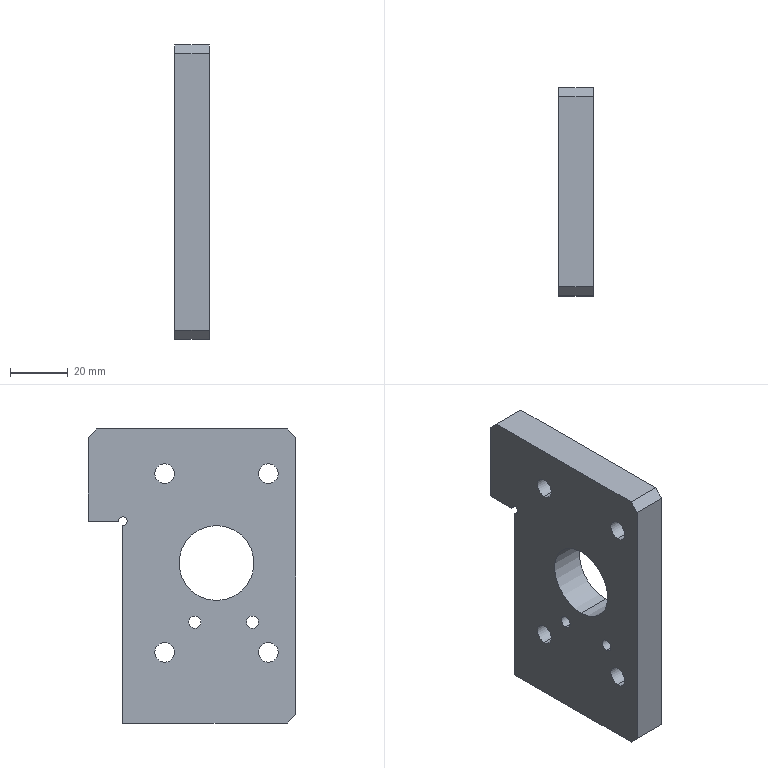Part | SolidWorks | features HoleWzd 3, Cut 2, Chamfer 1, Extrusion 1 | 1 solid | 34 faces | box 12 x 72 x 102 mm | volume 69020 mm3 | cylinder 19 | plane 11 | cone 4 | commonest cylinder face diameters 4.2 x8 6.8 x8 26 x2 3 x1
STEP:
#1=CARTESIAN_POINT('',(6.,47.6,-94.1));
#2=VERTEX_POINT('',#1);
#3=CARTESIAN_POINT('',(6.,47.6,-89.9));
#4=VERTEX_POINT('',#3);
#5=CARTESIAN_POINT('',(6.,47.6,-92.));
#6=DIRECTION('',(0.,1.,0.));
#7=DIRECTION('',(0.,0.,1.));
#8=AXIS2_PLACEMENT_3D('',#5,#6,#7);
#9=CIRCLE('',#8,2.1);
#10=EDGE_CURVE('',#2,#4,#9,.T.);
#11=ORIENTED_EDGE('',*,*,#10,.F.);
#12=CARTESIAN_POINT('',(6.,60.,-94.1));
#13=VERTEX_POINT('',#12);
#14=CARTESIAN_POINT('',(6.,60.,-94.1));
#15=DIRECTION('',(0.,1.,0.));
#16=VECTOR('',#15,1000.);
#17=LINE('',#14,#16);
#18=EDGE_CURVE('',#2,#13,#17,.T.);
#19=ORIENTED_EDGE('',*,*,#18,.T.);
#20=CARTESIAN_POINT('',(6.,60.,-89.9));
#21=VERTEX_POINT('',#20);
#22=CARTESIAN_POINT('',(6.,60.,-92.));
#23=DIRECTION('',(0.,1.,0.));
#24=DIRECTION('',(0.,0.,1.));
#25=AXIS2_PLACEMENT_3D('',#22,#23,#24);
#26=CIRCLE('',#25,2.1);
#27=EDGE_CURVE('',#13,#21,#26,.T.);
#28=ORIENTED_EDGE('',*,*,#27,.T.);
#29=CARTESIAN_POINT('',(6.,60.,-89.9));
#30=DIRECTION('',(0.,1.,0.));
#31=VECTOR('',#30,1000.);
#32=LINE('',#29,#31);
#33=EDGE_CURVE('',#4,#21,#32,.T.);
#34=ORIENTED_EDGE('',*,*,#33,.F.);
#35=EDGE_LOOP('',(#11,#19,#28,#34));
#36=FACE_OUTER_BOUND('',#35,.T.);
#37=CARTESIAN_POINT('',(6.,60.,-92.));
#38=DIRECTION('',(0.,1.,0.));
#39=DIRECTION('',(0.,0.,1.));
#40=AXIS2_PLACEMENT_3D('',#37,#38,#39);
#41=CYLINDRICAL_SURFACE('',#40,2.1);
#42=ADVANCED_FACE('',(#36),#41,.F.);
#43=CARTESIAN_POINT('',(6.,46.338,-92.));
#44=VERTEX_POINT('',#43);
#45=CARTESIAN_POINT('',(6.,47.6,-89.9));
#46=DIRECTION('',(0.,0.515,0.8572));
#47=VECTOR('',#46,1000.);
#48=LINE('',#45,#47);
#49=EDGE_CURVE('',#44,#4,#48,.T.);
#50=ORIENTED_EDGE('',*,*,#49,.F.);
#51=CARTESIAN_POINT('',(6.,47.6,-94.1));
#52=DIRECTION('',(0.,0.515,-0.8572));
#53=VECTOR('',#52,1000.);
#54=LINE('',#51,#53);
#55=EDGE_CURVE('',#44,#2,#54,.T.);
#56=ORIENTED_EDGE('',*,*,#55,.T.);
#57=ORIENTED_EDGE('',*,*,#10,.T.);
#58=EDGE_LOOP('',(#50,#56,#57));
#59=FACE_OUTER_BOUND('',#58,.T.);
#60=CARTESIAN_POINT('',(6.,47.6,-92.));
#61=DIRECTION('',(0.,1.,0.));
#62=DIRECTION('',(0.,0.,1.));
#63=AXIS2_PLACEMENT_3D('',#60,#61,#62);
#64=CONICAL_SURFACE('',#63,2.1,1.03);
#65=ADVANCED_FACE('',(#59),#64,.F.);
#66=CARTESIAN_POINT('',(6.,47.6,-44.1));
#67=VERTEX_POINT('',#66);
#68=CARTESIAN_POINT('',(6.,47.6,-39.9));
#69=VERTEX_POINT('',#68);
#70=CARTESIAN_POINT('',(6.,47.6,-42.));
#71=DIRECTION('',(0.,1.,0.));
#72=DIRECTION('',(0.,0.,1.));
#73=AXIS2_PLACEMENT_3D('',#70,#71,#72);
#74=CIRCLE('',#73,2.1);
#75=EDGE_CURVE('',#67,#69,#74,.T.);
#76=ORIENTED_EDGE('',*,*,#75,.F.);
#77=CARTESIAN_POINT('',(6.,60.,-44.1));
#78=VERTEX_POINT('',#77);
#79=CARTESIAN_POINT('',(6.,60.,-44.1));
#80=DIRECTION('',(0.,1.,0.));
#81=VECTOR('',#80,1000.);
#82=LINE('',#79,#81);
#83=EDGE_CURVE('',#67,#78,#82,.T.);
#84=ORIENTED_EDGE('',*,*,#83,.T.);
#85=CARTESIAN_POINT('',(6.,60.,-39.9));
#86=VERTEX_POINT('',#85);
#87=CARTESIAN_POINT('',(6.,60.,-42.));
#88=DIRECTION('',(0.,1.,0.));
#89=DIRECTION('',(0.,0.,1.));
#90=AXIS2_PLACEMENT_3D('',#87,#88,#89);
#91=CIRCLE('',#90,2.1);
#92=EDGE_CURVE('',#78,#86,#91,.T.);
#93=ORIENTED_EDGE('',*,*,#92,.T.);
#94=CARTESIAN_POINT('',(6.,60.,-39.9));
#95=DIRECTION('',(0.,1.,0.));
#96=VECTOR('',#95,1000.);
#97=LINE('',#94,#96);
#98=EDGE_CURVE('',#69,#86,#97,.T.);
#99=ORIENTED_EDGE('',*,*,#98,.F.);
#100=EDGE_LOOP('',(#76,#84,#93,#99));
#101=FACE_OUTER_BOUND('',#100,.T.);
#102=CARTESIAN_POINT('',(6.,60.,-42.));
#103=DIRECTION('',(0.,1.,0.));
#104=DIRECTION('',(0.,0.,1.));
#105=AXIS2_PLACEMENT_3D('',#102,#103,#104);
#106=CYLINDRICAL_SURFACE('',#105,2.1);
#107=ADVANCED_FACE('',(#101),#106,.F.);
#108=CARTESIAN_POINT('',(6.,46.338,-42.));
#109=VERTEX_POINT('',#108);
#110=CARTESIAN_POINT('',(6.,47.6,-39.9));
#111=DIRECTION('',(0.,0.515,0.8572));
#112=VECTOR('',#111,1000.);
#113=LINE('',#110,#112);
#114=EDGE_CURVE('',#109,#69,#113,.T.);
#115=ORIENTED_EDGE('',*,*,#114,.F.);
#116=CARTESIAN_POINT('',(6.,47.6,-44.1));
#117=DIRECTION('',(0.,0.515,-0.8572));
#118=VECTOR('',#117,1000.);
#119=LINE('',#116,#118);
#120=EDGE_CURVE('',#109,#67,#119,.T.);
#121=ORIENTED_EDGE('',*,*,#120,.T.);
#122=ORIENTED_EDGE('',*,*,#75,.T.);
#123=EDGE_LOOP('',(#115,#121,#122));
#124=FACE_OUTER_BOUND('',#123,.T.);
#125=CARTESIAN_POINT('',(6.,47.6,-42.));
#126=DIRECTION('',(0.,1.,0.));
#127=DIRECTION('',(0.,0.,1.));
#128=AXIS2_PLACEMENT_3D('',#125,#126,#127);
#129=CONICAL_SURFACE('',#128,2.1,1.03);
#130=ADVANCED_FACE('',(#124),#129,.F.);
#131=CARTESIAN_POINT('',(0.,35.,-64.9));
#132=VERTEX_POINT('',#131);
#133=CARTESIAN_POINT('',(0.,35.,-69.1));
#134=VERTEX_POINT('',#133);
#135=CARTESIAN_POINT('',(0.,35.,-67.));
#136=DIRECTION('',(1.,0.,0.));
#137=DIRECTION('',(0.,0.,-1.));
#138=AXIS2_PLACEMENT_3D('',#135,#136,#137);
#139=CIRCLE('',#138,2.1);
#140=EDGE_CURVE('',#132,#134,#139,.T.);
#141=ORIENTED_EDGE('',*,*,#140,.F.);
#142=CARTESIAN_POINT('',(12.,35.,-64.9));
#143=VERTEX_POINT('',#142);
#144=CARTESIAN_POINT('',(12.,35.,-64.9));
#145=DIRECTION('',(1.,0.,0.));
#146=VECTOR('',#145,1000.);
#147=LINE('',#144,#146);
#148=EDGE_CURVE('',#132,#143,#147,.T.);
#149=ORIENTED_EDGE('',*,*,#148,.T.);
#150=CARTESIAN_POINT('',(12.,35.,-69.1));
#151=VERTEX_POINT('',#150);
#152=CARTESIAN_POINT('',(12.,35.,-67.));
#153=DIRECTION('',(1.,0.,0.));
#154=DIRECTION('',(0.,0.,-1.));
#155=AXIS2_PLACEMENT_3D('',#152,#153,#154);
#156=CIRCLE('',#155,2.1);
#157=EDGE_CURVE('',#143,#151,#156,.T.);
#158=ORIENTED_EDGE('',*,*,#157,.T.);
#159=CARTESIAN_POINT('',(12.,35.,-69.1));
#160=DIRECTION('',(1.,0.,0.));
#161=VECTOR('',#160,1000.);
#162=LINE('',#159,#161);
#163=EDGE_CURVE('',#134,#151,#162,.T.);
#164=ORIENTED_EDGE('',*,*,#163,.F.);
#165=EDGE_LOOP('',(#141,#149,#158,#164));
#166=FACE_OUTER_BOUND('',#165,.T.);
#167=CARTESIAN_POINT('',(12.,35.,-67.));
#168=DIRECTION('',(1.,0.,0.));
#169=DIRECTION('',(0.,0.,-1.));
#170=AXIS2_PLACEMENT_3D('',#167,#168,#169);
#171=CYLINDRICAL_SURFACE('',#170,2.1);
#172=ADVANCED_FACE('',(#166),#171,.F.);
#173=CARTESIAN_POINT('',(0.,15.,-64.9));
#174=VERTEX_POINT('',#173);
#175=CARTESIAN_POINT('',(0.,15.,-69.1));
#176=VERTEX_POINT('',#175);
#177=CARTESIAN_POINT('',(0.,15.,-67.));
#178=DIRECTION('',(1.,0.,0.));
#179=DIRECTION('',(0.,0.,-1.));
#180=AXIS2_PLACEMENT_3D('',#177,#178,#179);
#181=CIRCLE('',#180,2.1);
#182=EDGE_CURVE('',#174,#176,#181,.T.);
#183=ORIENTED_EDGE('',*,*,#182,.F.);
#184=CARTESIAN_POINT('',(12.,15.,-64.9));
#185=VERTEX_POINT('',#184);
#186=CARTESIAN_POINT('',(12.,15.,-64.9));
#187=DIRECTION('',(1.,0.,0.));
#188=VECTOR('',#187,1000.);
#189=LINE('',#186,#188);
#190=EDGE_CURVE('',#174,#185,#189,.T.);
#191=ORIENTED_EDGE('',*,*,#190,.T.);
#192=CARTESIAN_POINT('',(12.,15.,-69.1));
#193=VERTEX_POINT('',#192);
#194=CARTESIAN_POINT('',(12.,15.,-67.));
#195=DIRECTION('',(1.,0.,0.));
#196=DIRECTION('',(0.,0.,-1.));
#197=AXIS2_PLACEMENT_3D('',#194,#195,#196);
#198=CIRCLE('',#197,2.1);
#199=EDGE_CURVE('',#185,#193,#198,.T.);
#200=ORIENTED_EDGE('',*,*,#199,.T.);
#201=CARTESIAN_POINT('',(12.,15.,-69.1));
#202=DIRECTION('',(1.,0.,0.));
#203=VECTOR('',#202,1000.);
#204=LINE('',#201,#203);
#205=EDGE_CURVE('',#176,#193,#204,.T.);
#206=ORIENTED_EDGE('',*,*,#205,.F.);
#207=EDGE_LOOP('',(#183,#191,#200,#206));
#208=FACE_OUTER_BOUND('',#207,.T.);
#209=CARTESIAN_POINT('',(12.,15.,-67.));
#210=DIRECTION('',(1.,0.,0.));
#211=DIRECTION('',(0.,0.,-1.));
#212=AXIS2_PLACEMENT_3D('',#209,#210,#211);
#213=CYLINDRICAL_SURFACE('',#212,2.1);
#214=ADVANCED_FACE('',(#208),#213,.F.);
#215=CARTESIAN_POINT('',(12.,45.5,-74.1));
#216=VERTEX_POINT('',#215);
#217=CARTESIAN_POINT('',(12.,45.5,-80.9));
#218=VERTEX_POINT('',#217);
#219=CARTESIAN_POINT('',(12.,45.5,-77.5));
#220=DIRECTION('',(1.,0.,0.));
#221=DIRECTION('',(0.,0.,-1.));
#222=AXIS2_PLACEMENT_3D('',#219,#220,#221);
#223=CIRCLE('',#222,3.4);
#224=EDGE_CURVE('',#216,#218,#223,.T.);
#225=ORIENTED_EDGE('',*,*,#224,.T.);
#226=CARTESIAN_POINT('',(0.,45.5,-80.9));
#227=VERTEX_POINT('',#226);
#228=CARTESIAN_POINT('',(0.,45.5,-80.9));
#229=DIRECTION('',(-1.,0.,0.));
#230=VECTOR('',#229,1000.);
#231=LINE('',#228,#230);
#232=EDGE_CURVE('',#218,#227,#231,.T.);
#233=ORIENTED_EDGE('',*,*,#232,.T.);
#234=CARTESIAN_POINT('',(0.,45.5,-74.1));
#235=VERTEX_POINT('',#234);
#236=CARTESIAN_POINT('',(0.,45.5,-77.5));
#237=DIRECTION('',(-1.,0.,0.));
#238=DIRECTION('',(0.,0.,1.));
#239=AXIS2_PLACEMENT_3D('',#236,#237,#238);
#240=CIRCLE('',#239,3.4);
#241=EDGE_CURVE('',#227,#235,#240,.T.);
#242=ORIENTED_EDGE('',*,*,#241,.T.);
#243=CARTESIAN_POINT('',(0.,45.5,-74.1));
#244=DIRECTION('',(-1.,0.,0.));
#245=VECTOR('',#244,1000.);
#246=LINE('',#243,#245);
#247=EDGE_CURVE('',#216,#235,#246,.T.);
#248=ORIENTED_EDGE('',*,*,#247,.F.);
#249=EDGE_LOOP('',(#225,#233,#242,#248));
#250=FACE_OUTER_BOUND('',#249,.T.);
#251=CARTESIAN_POINT('',(0.,45.5,-77.5));
#252=DIRECTION('',(-1.,0.,0.));
#253=DIRECTION('',(0.,0.,1.));
#254=AXIS2_PLACEMENT_3D('',#251,#252,#253);
#255=CYLINDRICAL_SURFACE('',#254,3.4);
#256=ADVANCED_FACE('',(#250),#255,.F.);
#257=CARTESIAN_POINT('',(12.,9.5,-74.1));
#258=VERTEX_POINT('',#257);
#259=CARTESIAN_POINT('',(12.,9.5,-80.9));
#260=VERTEX_POINT('',#259);
#261=CARTESIAN_POINT('',(12.,9.5,-77.5));
#262=DIRECTION('',(1.,0.,0.));
#263=DIRECTION('',(0.,0.,-1.));
#264=AXIS2_PLACEMENT_3D('',#261,#262,#263);
#265=CIRCLE('',#264,3.4);
#266=EDGE_CURVE('',#258,#260,#265,.T.);
#267=ORIENTED_EDGE('',*,*,#266,.T.);
#268=CARTESIAN_POINT('',(0.,9.5,-80.9));
#269=VERTEX_POINT('',#268);
#270=CARTESIAN_POINT('',(0.,9.5,-80.9));
#271=DIRECTION('',(-1.,0.,0.));
#272=VECTOR('',#271,1000.);
#273=LINE('',#270,#272);
#274=EDGE_CURVE('',#260,#269,#273,.T.);
#275=ORIENTED_EDGE('',*,*,#274,.T.);
#276=CARTESIAN_POINT('',(0.,9.5,-74.1));
#277=VERTEX_POINT('',#276);
#278=CARTESIAN_POINT('',(0.,9.5,-77.5));
#279=DIRECTION('',(-1.,0.,0.));
#280=DIRECTION('',(0.,0.,1.));
#281=AXIS2_PLACEMENT_3D('',#278,#279,#280);
#282=CIRCLE('',#281,3.4);
#283=EDGE_CURVE('',#269,#277,#282,.T.);
#284=ORIENTED_EDGE('',*,*,#283,.T.);
#285=CARTESIAN_POINT('',(0.,9.5,-74.1));
#286=DIRECTION('',(-1.,0.,0.));
#287=VECTOR('',#286,1000.);
#288=LINE('',#285,#287);
#289=EDGE_CURVE('',#258,#277,#288,.T.);
#290=ORIENTED_EDGE('',*,*,#289,.F.);
#291=EDGE_LOOP('',(#267,#275,#284,#290));
#292=FACE_OUTER_BOUND('',#291,.T.);
#293=CARTESIAN_POINT('',(0.,9.5,-77.5));
#294=DIRECTION('',(-1.,0.,0.));
#295=DIRECTION('',(0.,0.,1.));
#296=AXIS2_PLACEMENT_3D('',#293,#294,#295);
#297=CYLINDRICAL_SURFACE('',#296,3.4);
#298=ADVANCED_FACE('',(#292),#297,.F.);
#299=CARTESIAN_POINT('',(12.,9.5,-12.1));
#300=VERTEX_POINT('',#299);
#301=CARTESIAN_POINT('',(12.,9.5,-18.9));
#302=VERTEX_POINT('',#301);
#303=CARTESIAN_POINT('',(12.,9.5,-15.5));
#304=DIRECTION('',(1.,0.,0.));
#305=DIRECTION('',(0.,0.,-1.));
#306=AXIS2_PLACEMENT_3D('',#303,#304,#305);
#307=CIRCLE('',#306,3.4);
#308=EDGE_CURVE('',#300,#302,#307,.T.);
#309=ORIENTED_EDGE('',*,*,#308,.T.);
#310=CARTESIAN_POINT('',(0.,9.5,-18.9));
#311=VERTEX_POINT('',#310);
#312=CARTESIAN_POINT('',(0.,9.5,-18.9));
#313=DIRECTION('',(-1.,0.,0.));
#314=VECTOR('',#313,1000.);
#315=LINE('',#312,#314);
#316=EDGE_CURVE('',#302,#311,#315,.T.);
#317=ORIENTED_EDGE('',*,*,#316,.T.);
#318=CARTESIAN_POINT('',(0.,9.5,-12.1));
#319=VERTEX_POINT('',#318);
#320=CARTESIAN_POINT('',(0.,9.5,-15.5));
#321=DIRECTION('',(-1.,0.,0.));
#322=DIRECTION('',(0.,0.,1.));
#323=AXIS2_PLACEMENT_3D('',#320,#321,#322);
#324=CIRCLE('',#323,3.4);
#325=EDGE_CURVE('',#311,#319,#324,.T.);
#326=ORIENTED_EDGE('',*,*,#325,.T.);
#327=CARTESIAN_POINT('',(0.,9.5,-12.1));
#328=DIRECTION('',(-1.,0.,0.));
#329=VECTOR('',#328,1000.);
#330=LINE('',#327,#329);
#331=EDGE_CURVE('',#300,#319,#330,.T.);
#332=ORIENTED_EDGE('',*,*,#331,.F.);
#333=EDGE_LOOP('',(#309,#317,#326,#332));
#334=FACE_OUTER_BOUND('',#333,.T.);
#335=CARTESIAN_POINT('',(0.,9.5,-15.5));
#336=DIRECTION('',(-1.,0.,0.));
#337=DIRECTION('',(0.,0.,1.));
#338=AXIS2_PLACEMENT_3D('',#335,#336,#337);
#339=CYLINDRICAL_SURFACE('',#338,3.4);
#340=ADVANCED_FACE('',(#334),#339,.F.);
#341=CARTESIAN_POINT('',(12.,45.5,-12.1));
#342=VERTEX_POINT('',#341);
#343=CARTESIAN_POINT('',(12.,45.5,-18.9));
#344=VERTEX_POINT('',#343);
#345=CARTESIAN_POINT('',(12.,45.5,-15.5));
#346=DIRECTION('',(1.,0.,0.));
#347=DIRECTION('',(0.,0.,-1.));
#348=AXIS2_PLACEMENT_3D('',#345,#346,#347);
#349=CIRCLE('',#348,3.4);
#350=EDGE_CURVE('',#342,#344,#349,.T.);
#351=ORIENTED_EDGE('',*,*,#350,.T.);
#352=CARTESIAN_POINT('',(0.,45.5,-18.9));
#353=VERTEX_POINT('',#352);
#354=CARTESIAN_POINT('',(0.,45.5,-18.9));
#355=DIRECTION('',(-1.,0.,0.));
#356=VECTOR('',#355,1000.);
#357=LINE('',#354,#356);
#358=EDGE_CURVE('',#344,#353,#357,.T.);
#359=ORIENTED_EDGE('',*,*,#358,.T.);
#360=CARTESIAN_POINT('',(0.,45.5,-12.1));
#361=VERTEX_POINT('',#360);
#362=CARTESIAN_POINT('',(0.,45.5,-15.5));
#363=DIRECTION('',(-1.,0.,0.));
#364=DIRECTION('',(0.,0.,1.));
#365=AXIS2_PLACEMENT_3D('',#362,#363,#364);
#366=CIRCLE('',#365,3.4);
#367=EDGE_CURVE('',#353,#361,#366,.T.);
#368=ORIENTED_EDGE('',*,*,#367,.T.);
#369=CARTESIAN_POINT('',(0.,45.5,-12.1));
#370=DIRECTION('',(-1.,0.,0.));
#371=VECTOR('',#370,1000.);
#372=LINE('',#369,#371);
#373=EDGE_CURVE('',#342,#361,#372,.T.);
#374=ORIENTED_EDGE('',*,*,#373,.F.);
#375=EDGE_LOOP('',(#351,#359,#368,#374));
#376=FACE_OUTER_BOUND('',#375,.T.);
#377=CARTESIAN_POINT('',(0.,45.5,-15.5));
#378=DIRECTION('',(-1.,0.,0.));
#379=DIRECTION('',(0.,0.,1.));
#380=AXIS2_PLACEMENT_3D('',#377,#378,#379);
#381=CYLINDRICAL_SURFACE('',#380,3.4);
#382=ADVANCED_FACE('',(#376),#381,.F.);
#383=CARTESIAN_POINT('',(0.,27.5,-33.5));
#384=VERTEX_POINT('',#383);
#385=CARTESIAN_POINT('',(0.,27.5,-59.5));
#386=VERTEX_POINT('',#385);
#387=CARTESIAN_POINT('',(0.,27.5,-46.5));
#388=DIRECTION('',(1.,0.,0.));
#389=DIRECTION('',(0.,0.,-1.));
#390=AXIS2_PLACEMENT_3D('',#387,#388,#389);
#391=CIRCLE('',#390,13.);
#392=EDGE_CURVE('',#384,#386,#391,.T.);
#393=ORIENTED_EDGE('',*,*,#392,.F.);
#394=CARTESIAN_POINT('',(12.,27.5,-33.5));
#395=VERTEX_POINT('',#394);
#396=CARTESIAN_POINT('',(0.,27.5,-33.5));
#397=DIRECTION('',(1.,0.,0.));
#398=VECTOR('',#397,1000.);
#399=LINE('',#396,#398);
#400=EDGE_CURVE('',#384,#395,#399,.T.);
#401=ORIENTED_EDGE('',*,*,#400,.T.);
#402=CARTESIAN_POINT('',(12.,27.5,-59.5));
#403=VERTEX_POINT('',#402);
#404=CARTESIAN_POINT('',(12.,27.5,-46.5));
#405=DIRECTION('',(1.,0.,0.));
#406=DIRECTION('',(0.,0.,-1.));
#407=AXIS2_PLACEMENT_3D('',#404,#405,#406);
#408=CIRCLE('',#407,13.);
#409=EDGE_CURVE('',#395,#403,#408,.T.);
#410=ORIENTED_EDGE('',*,*,#409,.T.);
#411=CARTESIAN_POINT('',(0.,27.5,-59.5));
#412=DIRECTION('',(1.,0.,0.));
#413=VECTOR('',#412,1000.);
#414=LINE('',#411,#413);
#415=EDGE_CURVE('',#386,#403,#414,.T.);
#416=ORIENTED_EDGE('',*,*,#415,.F.);
#417=EDGE_LOOP('',(#393,#401,#410,#416));
#418=FACE_OUTER_BOUND('',#417,.T.);
#419=CARTESIAN_POINT('',(0.,27.5,-46.5));
#420=DIRECTION('',(1.,0.,0.));
#421=DIRECTION('',(0.,0.,-1.));
#422=AXIS2_PLACEMENT_3D('',#419,#420,#421);
#423=CYLINDRICAL_SURFACE('',#422,13.);
#424=ADVANCED_FACE('',(#418),#423,.F.);
#425=CARTESIAN_POINT('',(12.,69.,0.));
#426=VERTEX_POINT('',#425);
#427=CARTESIAN_POINT('',(12.,3.,0.));
#428=VERTEX_POINT('',#427);
#429=CARTESIAN_POINT('',(12.,72.,0.));
#430=DIRECTION('',(0.,-1.,0.));
#431=VECTOR('',#430,1000.);
#432=LINE('',#429,#431);
#433=EDGE_CURVE('',#426,#428,#432,.T.);
#434=ORIENTED_EDGE('',*,*,#433,.F.);
#435=CARTESIAN_POINT('',(0.,69.,0.));
#436=VERTEX_POINT('',#435);
#437=CARTESIAN_POINT('',(12.,69.,0.));
#438=DIRECTION('',(-1.,0.,0.));
#439=VECTOR('',#438,1000.);
#440=LINE('',#437,#439);
#441=EDGE_CURVE('',#426,#436,#440,.T.);
#442=ORIENTED_EDGE('',*,*,#441,.T.);
#443=CARTESIAN_POINT('',(0.,3.,0.));
#444=VERTEX_POINT('',#443);
#445=CARTESIAN_POINT('',(0.,72.,0.));
#446=DIRECTION('',(0.,-1.,0.));
#447=VECTOR('',#446,1000.);
#448=LINE('',#445,#447);
#449=EDGE_CURVE('',#436,#444,#448,.T.);
#450=ORIENTED_EDGE('',*,*,#449,.T.);
#451=CARTESIAN_POINT('',(12.,3.,0.));
#452=DIRECTION('',(1.,0.,0.));
#453=VECTOR('',#452,1000.);
#454=LINE('',#451,#453);
#455=EDGE_CURVE('',#444,#428,#454,.T.);
#456=ORIENTED_EDGE('',*,*,#455,.T.);
#457=EDGE_LOOP('',(#434,#442,#450,#456));
#458=FACE_OUTER_BOUND('',#457,.T.);
#459=CARTESIAN_POINT('',(12.,72.,0.));
#460=DIRECTION('',(0.,0.,-1.));
#461=DIRECTION('',(0.,1.,0.));
#462=AXIS2_PLACEMENT_3D('',#459,#460,#461);
#463=PLANE('',#462);
#464=ADVANCED_FACE('',(#458),#463,.F.);
#465=CARTESIAN_POINT('',(0.,0.,-3.));
#466=VERTEX_POINT('',#465);
#467=CARTESIAN_POINT('',(0.,0.,-99.));
#468=VERTEX_POINT('',#467);
#469=CARTESIAN_POINT('',(0.,0.,0.));
#470=DIRECTION('',(0.,0.,-1.));
#471=VECTOR('',#470,1000.);
#472=LINE('',#469,#471);
#473=EDGE_CURVE('',#466,#468,#472,.T.);
#474=ORIENTED_EDGE('',*,*,#473,.T.);
#475=CARTESIAN_POINT('',(12.,0.,-99.));
#476=VERTEX_POINT('',#475);
#477=CARTESIAN_POINT('',(12.,0.,-99.));
#478=DIRECTION('',(1.,0.,0.));
#479=VECTOR('',#478,1000.);
#480=LINE('',#477,#479);
#481=EDGE_CURVE('',#468,#476,#480,.T.);
#482=ORIENTED_EDGE('',*,*,#481,.T.);
#483=CARTESIAN_POINT('',(12.,0.,-3.));
#484=VERTEX_POINT('',#483);
#485=CARTESIAN_POINT('',(12.,0.,0.));
#486=DIRECTION('',(0.,0.,-1.));
#487=VECTOR('',#486,1000.);
#488=LINE('',#485,#487);
#489=EDGE_CURVE('',#484,#476,#488,.T.);
#490=ORIENTED_EDGE('',*,*,#489,.F.);
#491=CARTESIAN_POINT('',(12.,0.,-3.));
#492=DIRECTION('',(-1.,0.,0.));
#493=VECTOR('',#492,1000.);
#494=LINE('',#491,#493);
#495=EDGE_CURVE('',#484,#466,#494,.T.);
#496=ORIENTED_EDGE('',*,*,#495,.T.);
#497=EDGE_LOOP('',(#474,#482,#490,#496));
#498=FACE_OUTER_BOUND('',#497,.T.);
#499=CARTESIAN_POINT('',(12.,0.,0.));
#500=DIRECTION('',(0.,1.,0.));
#501=DIRECTION('',(0.,0.,1.));
#502=AXIS2_PLACEMENT_3D('',#499,#500,#501);
#503=PLANE('',#502);
#504=ADVANCED_FACE('',(#498),#503,.F.);
#505=CARTESIAN_POINT('',(12.,3.,-102.));
#506=VERTEX_POINT('',#505);
#507=CARTESIAN_POINT('',(12.,60.,-102.));
#508=VERTEX_POINT('',#507);
#509=CARTESIAN_POINT('',(12.,0.,-102.));
#510=DIRECTION('',(0.,1.,0.));
#511=VECTOR('',#510,1000.);
#512=LINE('',#509,#511);
#513=EDGE_CURVE('',#506,#508,#512,.T.);
#514=ORIENTED_EDGE('',*,*,#513,.F.);
#515=CARTESIAN_POINT('',(0.,3.,-102.));
#516=VERTEX_POINT('',#515);
#517=CARTESIAN_POINT('',(12.,3.,-102.));
#518=DIRECTION('',(-1.,0.,0.));
#519=VECTOR('',#518,1000.);
#520=LINE('',#517,#519);
#521=EDGE_CURVE('',#506,#516,#520,.T.);
#522=ORIENTED_EDGE('',*,*,#521,.T.);
#523=CARTESIAN_POINT('',(0.,60.,-102.));
#524=VERTEX_POINT('',#523);
#525=CARTESIAN_POINT('',(0.,0.,-102.));
#526=DIRECTION('',(0.,1.,0.));
#527=VECTOR('',#526,1000.);
#528=LINE('',#525,#527);
#529=EDGE_CURVE('',#516,#524,#528,.T.);
#530=ORIENTED_EDGE('',*,*,#529,.T.);
#531=CARTESIAN_POINT('',(12.,60.,-102.));
#532=DIRECTION('',(-1.,0.,0.));
#533=VECTOR('',#532,1000.);
#534=LINE('',#531,#533);
#535=EDGE_CURVE('',#508,#524,#534,.T.);
#536=ORIENTED_EDGE('',*,*,#535,.F.);
#537=EDGE_LOOP('',(#514,#522,#530,#536));
#538=FACE_OUTER_BOUND('',#537,.T.);
#539=CARTESIAN_POINT('',(12.,0.,-102.));
#540=DIRECTION('',(0.,0.,1.));
#541=DIRECTION('',(1.,0.,0.));
#542=AXIS2_PLACEMENT_3D('',#539,#540,#541);
#543=PLANE('',#542);
#544=ADVANCED_FACE('',(#538),#543,.F.);
#545=CARTESIAN_POINT('',(6.,60.,-92.));
#546=DIRECTION('',(0.,1.,0.));
#547=DIRECTION('',(0.,0.,1.));
#548=AXIS2_PLACEMENT_3D('',#545,#546,#547);
#549=CIRCLE('',#548,2.1);
#550=EDGE_CURVE('',#21,#13,#549,.T.);
#551=ORIENTED_EDGE('',*,*,#550,.F.);
#552=ORIENTED_EDGE('',*,*,#27,.F.);
#553=EDGE_LOOP('',(#551,#552));
#554=FACE_BOUND('',#553,.T.);
#555=CARTESIAN_POINT('',(6.,60.,-42.));
#556=DIRECTION('',(0.,1.,0.));
#557=DIRECTION('',(0.,0.,1.));
#558=AXIS2_PLACEMENT_3D('',#555,#556,#557);
#559=CIRCLE('',#558,2.1);
#560=EDGE_CURVE('',#86,#78,#559,.T.);
#561=ORIENTED_EDGE('',*,*,#560,.F.);
#562=ORIENTED_EDGE('',*,*,#92,.F.);
#563=EDGE_LOOP('',(#561,#562));
#564=FACE_BOUND('',#563,.T.);
#565=CARTESIAN_POINT('',(0.,60.,-33.5));
#566=VERTEX_POINT('',#565);
#567=CARTESIAN_POINT('',(0.,60.,-102.));
#568=DIRECTION('',(0.,0.,1.));
#569=VECTOR('',#568,1000.);
#570=LINE('',#567,#569);
#571=EDGE_CURVE('',#524,#566,#570,.T.);
#572=ORIENTED_EDGE('',*,*,#571,.T.);
#573=CARTESIAN_POINT('',(12.,60.,-33.5));
#574=VERTEX_POINT('',#573);
#575=CARTESIAN_POINT('',(0.,60.,-33.5));
#576=DIRECTION('',(1.,0.,0.));
#577=VECTOR('',#576,1000.);
#578=LINE('',#575,#577);
#579=EDGE_CURVE('',#566,#574,#578,.T.);
#580=ORIENTED_EDGE('',*,*,#579,.T.);
#581=CARTESIAN_POINT('',(12.,60.,-102.));
#582=DIRECTION('',(0.,0.,1.));
#583=VECTOR('',#582,1000.);
#584=LINE('',#581,#583);
#585=EDGE_CURVE('',#508,#574,#584,.T.);
#586=ORIENTED_EDGE('',*,*,#585,.F.);
#587=ORIENTED_EDGE('',*,*,#535,.T.);
#588=EDGE_LOOP('',(#572,#580,#586,#587));
#589=FACE_OUTER_BOUND('',#588,.T.);
#590=CARTESIAN_POINT('',(12.,60.,-102.));
#591=DIRECTION('',(0.,-1.,0.));
#592=DIRECTION('',(0.,0.,-1.));
#593=AXIS2_PLACEMENT_3D('',#590,#591,#592);
#594=PLANE('',#593);
#595=ADVANCED_FACE('',(#554,#564,#589),#594,.F.);
#596=CARTESIAN_POINT('',(12.,61.5,-32.));
#597=VERTEX_POINT('',#596);
#598=CARTESIAN_POINT('',(12.,72.,-32.));
#599=VERTEX_POINT('',#598);
#600=CARTESIAN_POINT('',(12.,60.,-32.));
#601=DIRECTION('',(0.,1.,0.));
#602=VECTOR('',#601,1000.);
#603=LINE('',#600,#602);
#604=EDGE_CURVE('',#597,#599,#603,.T.);
#605=ORIENTED_EDGE('',*,*,#604,.F.);
#606=CARTESIAN_POINT('',(0.,61.5,-32.));
#607=VERTEX_POINT('',#606);
#608=CARTESIAN_POINT('',(0.,61.5,-32.));
#609=DIRECTION('',(-1.,0.,0.));
#610=VECTOR('',#609,1000.);
#611=LINE('',#608,#610);
#612=EDGE_CURVE('',#597,#607,#611,.T.);
#613=ORIENTED_EDGE('',*,*,#612,.T.);
#614=CARTESIAN_POINT('',(0.,72.,-32.));
#615=VERTEX_POINT('',#614);
#616=CARTESIAN_POINT('',(0.,60.,-32.));
#617=DIRECTION('',(0.,1.,0.));
#618=VECTOR('',#617,1000.);
#619=LINE('',#616,#618);
#620=EDGE_CURVE('',#607,#615,#619,.T.);
#621=ORIENTED_EDGE('',*,*,#620,.T.);
#622=CARTESIAN_POINT('',(12.,72.,-32.));
#623=DIRECTION('',(-1.,0.,0.));
#624=VECTOR('',#623,1000.);
#625=LINE('',#622,#624);
#626=EDGE_CURVE('',#599,#615,#625,.T.);
#627=ORIENTED_EDGE('',*,*,#626,.F.);
#628=EDGE_LOOP('',(#605,#613,#621,#627));
#629=FACE_OUTER_BOUND('',#628,.T.);
#630=CARTESIAN_POINT('',(12.,60.,-32.));
#631=DIRECTION('',(0.,0.,1.));
#632=DIRECTION('',(1.,0.,0.));
#633=AXIS2_PLACEMENT_3D('',#630,#631,#632);
#634=PLANE('',#633);
#635=ADVANCED_FACE('',(#629),#634,.F.);
#636=CARTESIAN_POINT('',(0.,72.,-3.));
#637=VERTEX_POINT('',#636);
#638=CARTESIAN_POINT('',(0.,72.,-32.));
#639=DIRECTION('',(0.,0.,1.));
#640=VECTOR('',#639,1000.);
#641=LINE('',#638,#640);
#642=EDGE_CURVE('',#615,#637,#641,.T.);
#643=ORIENTED_EDGE('',*,*,#642,.T.);
#644=CARTESIAN_POINT('',(12.,72.,-3.));
#645=VERTEX_POINT('',#644);
#646=CARTESIAN_POINT('',(12.,72.,-3.));
#647=DIRECTION('',(1.,0.,0.));
#648=VECTOR('',#647,1000.);
#649=LINE('',#646,#648);
#650=EDGE_CURVE('',#637,#645,#649,.T.);
#651=ORIENTED_EDGE('',*,*,#650,.T.);
#652=CARTESIAN_POINT('',(12.,72.,-32.));
#653=DIRECTION('',(0.,0.,1.));
#654=VECTOR('',#653,1000.);
#655=LINE('',#652,#654);
#656=EDGE_CURVE('',#599,#645,#655,.T.);
#657=ORIENTED_EDGE('',*,*,#656,.F.);
#658=ORIENTED_EDGE('',*,*,#626,.T.);
#659=EDGE_LOOP('',(#643,#651,#657,#658));
#660=FACE_OUTER_BOUND('',#659,.T.);
#661=CARTESIAN_POINT('',(12.,72.,-32.));
#662=DIRECTION('',(0.,-1.,0.));
#663=DIRECTION('',(0.,0.,-1.));
#664=AXIS2_PLACEMENT_3D('',#661,#662,#663);
#665=PLANE('',#664);
#666=ADVANCED_FACE('',(#660),#665,.F.);
#667=CARTESIAN_POINT('',(12.,60.,-32.));
#668=DIRECTION('',(1.,0.,0.));
#669=DIRECTION('',(0.,0.,-1.));
#670=AXIS2_PLACEMENT_3D('',#667,#668,#669);
#671=CIRCLE('',#670,1.5);
#672=EDGE_CURVE('',#597,#574,#671,.T.);
#673=ORIENTED_EDGE('',*,*,#672,.F.);
#674=ORIENTED_EDGE('',*,*,#604,.T.);
#675=ORIENTED_EDGE('',*,*,#656,.T.);
#676=CARTESIAN_POINT('',(12.,34.5,34.5));
#677=DIRECTION('',(0.,-0.7071,0.7071));
#678=VECTOR('',#677,1000.);
#679=LINE('',#676,#678);
#680=EDGE_CURVE('',#645,#426,#679,.T.);
#681=ORIENTED_EDGE('',*,*,#680,.T.);
#682=ORIENTED_EDGE('',*,*,#433,.T.);
#683=CARTESIAN_POINT('',(12.,1.5,-1.5));
#684=DIRECTION('',(0.,-0.7071,-0.7071));
#685=VECTOR('',#684,1000.);
#686=LINE('',#683,#685);
#687=EDGE_CURVE('',#428,#484,#686,.T.);
#688=ORIENTED_EDGE('',*,*,#687,.T.);
#689=ORIENTED_EDGE('',*,*,#489,.T.);
#690=CARTESIAN_POINT('',(12.,-49.5,-49.5));
#691=DIRECTION('',(0.,0.7071,-0.7071));
#692=VECTOR('',#691,1000.);
#693=LINE('',#690,#692);
#694=EDGE_CURVE('',#476,#506,#693,.T.);
#695=ORIENTED_EDGE('',*,*,#694,.T.);
#696=ORIENTED_EDGE('',*,*,#513,.T.);
#697=ORIENTED_EDGE('',*,*,#585,.T.);
#698=EDGE_LOOP('',(#673,#674,#675,#681,#682,#688,#689,#695,#696,#697));
#699=FACE_OUTER_BOUND('',#698,.T.);
#700=CARTESIAN_POINT('',(12.,35.,-67.));
#701=DIRECTION('',(1.,0.,0.));
#702=DIRECTION('',(0.,0.,-1.));
#703=AXIS2_PLACEMENT_3D('',#700,#701,#702);
#704=CIRCLE('',#703,2.1);
#705=EDGE_CURVE('',#151,#143,#704,.T.);
#706=ORIENTED_EDGE('',*,*,#705,.F.);
#707=ORIENTED_EDGE('',*,*,#157,.F.);
#708=EDGE_LOOP('',(#706,#707));
#709=FACE_BOUND('',#708,.T.);
#710=CARTESIAN_POINT('',(12.,15.,-67.));
#711=DIRECTION('',(1.,0.,0.));
#712=DIRECTION('',(0.,0.,-1.));
#713=AXIS2_PLACEMENT_3D('',#710,#711,#712);
#714=CIRCLE('',#713,2.1);
#715=EDGE_CURVE('',#193,#185,#714,.T.);
#716=ORIENTED_EDGE('',*,*,#715,.F.);
#717=ORIENTED_EDGE('',*,*,#199,.F.);
#718=EDGE_LOOP('',(#716,#717));
#719=FACE_BOUND('',#718,.T.);
#720=ORIENTED_EDGE('',*,*,#224,.F.);
#721=CARTESIAN_POINT('',(12.,45.5,-77.5));
#722=DIRECTION('',(1.,0.,0.));
#723=DIRECTION('',(0.,0.,-1.));
#724=AXIS2_PLACEMENT_3D('',#721,#722,#723);
#725=CIRCLE('',#724,3.4);
#726=EDGE_CURVE('',#218,#216,#725,.T.);
#727=ORIENTED_EDGE('',*,*,#726,.F.);
#728=EDGE_LOOP('',(#720,#727));
#729=FACE_BOUND('',#728,.T.);
#730=ORIENTED_EDGE('',*,*,#266,.F.);
#731=CARTESIAN_POINT('',(12.,9.5,-77.5));
#732=DIRECTION('',(1.,0.,0.));
#733=DIRECTION('',(0.,0.,-1.));
#734=AXIS2_PLACEMENT_3D('',#731,#732,#733);
#735=CIRCLE('',#734,3.4);
#736=EDGE_CURVE('',#260,#258,#735,.T.);
#737=ORIENTED_EDGE('',*,*,#736,.F.);
#738=EDGE_LOOP('',(#730,#737));
#739=FACE_BOUND('',#738,.T.);
#740=ORIENTED_EDGE('',*,*,#308,.F.);
#741=CARTESIAN_POINT('',(12.,9.5,-15.5));
#742=DIRECTION('',(1.,0.,0.));
#743=DIRECTION('',(0.,0.,-1.));
#744=AXIS2_PLACEMENT_3D('',#741,#742,#743);
#745=CIRCLE('',#744,3.4);
#746=EDGE_CURVE('',#302,#300,#745,.T.);
#747=ORIENTED_EDGE('',*,*,#746,.F.);
#748=EDGE_LOOP('',(#740,#747));
#749=FACE_BOUND('',#748,.T.);
#750=ORIENTED_EDGE('',*,*,#350,.F.);
#751=CARTESIAN_POINT('',(12.,45.5,-15.5));
#752=DIRECTION('',(1.,0.,0.));
#753=DIRECTION('',(0.,0.,-1.));
#754=AXIS2_PLACEMENT_3D('',#751,#752,#753);
#755=CIRCLE('',#754,3.4);
#756=EDGE_CURVE('',#344,#342,#755,.T.);
#757=ORIENTED_EDGE('',*,*,#756,.F.);
#758=EDGE_LOOP('',(#750,#757));
#759=FACE_BOUND('',#758,.T.);
#760=CARTESIAN_POINT('',(12.,27.5,-46.5));
#761=DIRECTION('',(1.,0.,0.));
#762=DIRECTION('',(0.,0.,-1.));
#763=AXIS2_PLACEMENT_3D('',#760,#761,#762);
#764=CIRCLE('',#763,13.);
#765=EDGE_CURVE('',#403,#395,#764,.T.);
#766=ORIENTED_EDGE('',*,*,#765,.F.);
#767=ORIENTED_EDGE('',*,*,#409,.F.);
#768=EDGE_LOOP('',(#766,#767));
#769=FACE_BOUND('',#768,.T.);
#770=CARTESIAN_POINT('',(12.,0.,0.));
#771=DIRECTION('',(1.,0.,0.));
#772=DIRECTION('',(0.,0.,-1.));
#773=AXIS2_PLACEMENT_3D('',#770,#771,#772);
#774=PLANE('',#773);
#775=ADVANCED_FACE('',(#699,#709,#719,#729,#739,#749,#759,#769),#774,.T.);
#776=CARTESIAN_POINT('',(0.,35.,-67.));
#777=DIRECTION('',(1.,0.,0.));
#778=DIRECTION('',(0.,0.,-1.));
#779=AXIS2_PLACEMENT_3D('',#776,#777,#778);
#780=CIRCLE('',#779,2.1);
#781=EDGE_CURVE('',#134,#132,#780,.T.);
#782=ORIENTED_EDGE('',*,*,#781,.T.);
#783=ORIENTED_EDGE('',*,*,#140,.T.);
#784=EDGE_LOOP('',(#782,#783));
#785=FACE_BOUND('',#784,.T.);
#786=CARTESIAN_POINT('',(0.,15.,-67.));
#787=DIRECTION('',(1.,0.,0.));
#788=DIRECTION('',(0.,0.,-1.));
#789=AXIS2_PLACEMENT_3D('',#786,#787,#788);
#790=CIRCLE('',#789,2.1);
#791=EDGE_CURVE('',#176,#174,#790,.T.);
#792=ORIENTED_EDGE('',*,*,#791,.T.);
#793=ORIENTED_EDGE('',*,*,#182,.T.);
#794=EDGE_LOOP('',(#792,#793));
#795=FACE_BOUND('',#794,.T.);
#796=CARTESIAN_POINT('',(0.,45.5,-77.5));
#797=DIRECTION('',(-1.,0.,0.));
#798=DIRECTION('',(0.,0.,1.));
#799=AXIS2_PLACEMENT_3D('',#796,#797,#798);
#800=CIRCLE('',#799,3.4);
#801=EDGE_CURVE('',#235,#227,#800,.T.);
#802=ORIENTED_EDGE('',*,*,#801,.F.);
#803=ORIENTED_EDGE('',*,*,#241,.F.);
#804=EDGE_LOOP('',(#802,#803));
#805=FACE_BOUND('',#804,.T.);
#806=CARTESIAN_POINT('',(0.,9.5,-77.5));
#807=DIRECTION('',(-1.,0.,0.));
#808=DIRECTION('',(0.,0.,1.));
#809=AXIS2_PLACEMENT_3D('',#806,#807,#808);
#810=CIRCLE('',#809,3.4);
#811=EDGE_CURVE('',#277,#269,#810,.T.);
#812=ORIENTED_EDGE('',*,*,#811,.F.);
#813=ORIENTED_EDGE('',*,*,#283,.F.);
#814=EDGE_LOOP('',(#812,#813));
#815=FACE_BOUND('',#814,.T.);
#816=CARTESIAN_POINT('',(0.,9.5,-15.5));
#817=DIRECTION('',(-1.,0.,0.));
#818=DIRECTION('',(0.,0.,1.));
#819=AXIS2_PLACEMENT_3D('',#816,#817,#818);
#820=CIRCLE('',#819,3.4);
#821=EDGE_CURVE('',#319,#311,#820,.T.);
#822=ORIENTED_EDGE('',*,*,#821,.F.);
#823=ORIENTED_EDGE('',*,*,#325,.F.);
#824=EDGE_LOOP('',(#822,#823));
#825=FACE_BOUND('',#824,.T.);
#826=CARTESIAN_POINT('',(0.,45.5,-15.5));
#827=DIRECTION('',(-1.,0.,0.));
#828=DIRECTION('',(0.,0.,1.));
#829=AXIS2_PLACEMENT_3D('',#826,#827,#828);
#830=CIRCLE('',#829,3.4);
#831=EDGE_CURVE('',#361,#353,#830,.T.);
#832=ORIENTED_EDGE('',*,*,#831,.F.);
#833=ORIENTED_EDGE('',*,*,#367,.F.);
#834=EDGE_LOOP('',(#832,#833));
#835=FACE_BOUND('',#834,.T.);
#836=CARTESIAN_POINT('',(0.,27.5,-46.5));
#837=DIRECTION('',(1.,0.,0.));
#838=DIRECTION('',(0.,0.,-1.));
#839=AXIS2_PLACEMENT_3D('',#836,#837,#838);
#840=CIRCLE('',#839,13.);
#841=EDGE_CURVE('',#386,#384,#840,.T.);
#842=ORIENTED_EDGE('',*,*,#841,.T.);
#843=ORIENTED_EDGE('',*,*,#392,.T.);
#844=EDGE_LOOP('',(#842,#843));
#845=FACE_BOUND('',#844,.T.);
#846=ORIENTED_EDGE('',*,*,#620,.F.);
#847=CARTESIAN_POINT('',(0.,60.,-32.));
#848=DIRECTION('',(1.,0.,0.));
#849=DIRECTION('',(0.,0.,-1.));
#850=AXIS2_PLACEMENT_3D('',#847,#848,#849);
#851=CIRCLE('',#850,1.5);
#852=EDGE_CURVE('',#607,#566,#851,.T.);
#853=ORIENTED_EDGE('',*,*,#852,.T.);
#854=ORIENTED_EDGE('',*,*,#571,.F.);
#855=ORIENTED_EDGE('',*,*,#529,.F.);
#856=CARTESIAN_POINT('',(0.,3.,-102.));
#857=DIRECTION('',(0.,-0.7071,0.7071));
#858=VECTOR('',#857,1000.);
#859=LINE('',#856,#858);
#860=EDGE_CURVE('',#516,#468,#859,.T.);
#861=ORIENTED_EDGE('',*,*,#860,.T.);
#862=ORIENTED_EDGE('',*,*,#473,.F.);
#863=CARTESIAN_POINT('',(0.,0.,-3.));
#864=DIRECTION('',(0.,0.7071,0.7071));
#865=VECTOR('',#864,1000.);
#866=LINE('',#863,#865);
#867=EDGE_CURVE('',#466,#444,#866,.T.);
#868=ORIENTED_EDGE('',*,*,#867,.T.);
#869=ORIENTED_EDGE('',*,*,#449,.F.);
#870=CARTESIAN_POINT('',(0.,69.,0.));
#871=DIRECTION('',(0.,0.7071,-0.7071));
#872=VECTOR('',#871,1000.);
#873=LINE('',#870,#872);
#874=EDGE_CURVE('',#436,#637,#873,.T.);
#875=ORIENTED_EDGE('',*,*,#874,.T.);
#876=ORIENTED_EDGE('',*,*,#642,.F.);
#877=EDGE_LOOP('',(#846,#853,#854,#855,#861,#862,#868,#869,#875,#876));
#878=FACE_OUTER_BOUND('',#877,.T.);
#879=CARTESIAN_POINT('',(0.,0.,0.));
#880=DIRECTION('',(1.,0.,0.));
#881=DIRECTION('',(0.,0.,-1.));
#882=AXIS2_PLACEMENT_3D('',#879,#880,#881);
#883=PLANE('',#882);
#884=ADVANCED_FACE('',(#785,#795,#805,#815,#825,#835,#845,#878),#883,.F.);
#885=ORIENTED_EDGE('',*,*,#400,.F.);
#886=ORIENTED_EDGE('',*,*,#841,.F.);
#887=ORIENTED_EDGE('',*,*,#415,.T.);
#888=ORIENTED_EDGE('',*,*,#765,.T.);
#889=EDGE_LOOP('',(#885,#886,#887,#888));
#890=FACE_OUTER_BOUND('',#889,.T.);
#891=CARTESIAN_POINT('',(0.,27.5,-46.5));
#892=DIRECTION('',(1.,0.,0.));
#893=DIRECTION('',(0.,0.,-1.));
#894=AXIS2_PLACEMENT_3D('',#891,#892,#893);
#895=CYLINDRICAL_SURFACE('',#894,13.);
#896=ADVANCED_FACE('',(#890),#895,.F.);
#897=ORIENTED_EDGE('',*,*,#358,.F.);
#898=ORIENTED_EDGE('',*,*,#756,.T.);
#899=ORIENTED_EDGE('',*,*,#373,.T.);
#900=ORIENTED_EDGE('',*,*,#831,.T.);
#901=EDGE_LOOP('',(#897,#898,#899,#900));
#902=FACE_OUTER_BOUND('',#901,.T.);
#903=CARTESIAN_POINT('',(0.,45.5,-15.5));
#904=DIRECTION('',(-1.,0.,0.));
#905=DIRECTION('',(0.,0.,1.));
#906=AXIS2_PLACEMENT_3D('',#903,#904,#905);
#907=CYLINDRICAL_SURFACE('',#906,3.4);
#908=ADVANCED_FACE('',(#902),#907,.F.);
#909=ORIENTED_EDGE('',*,*,#316,.F.);
#910=ORIENTED_EDGE('',*,*,#746,.T.);
#911=ORIENTED_EDGE('',*,*,#331,.T.);
#912=ORIENTED_EDGE('',*,*,#821,.T.);
#913=EDGE_LOOP('',(#909,#910,#911,#912));
#914=FACE_OUTER_BOUND('',#913,.T.);
#915=CARTESIAN_POINT('',(0.,9.5,-15.5));
#916=DIRECTION('',(-1.,0.,0.));
#917=DIRECTION('',(0.,0.,1.));
#918=AXIS2_PLACEMENT_3D('',#915,#916,#917);
#919=CYLINDRICAL_SURFACE('',#918,3.4);
#920=ADVANCED_FACE('',(#914),#919,.F.);
#921=ORIENTED_EDGE('',*,*,#274,.F.);
#922=ORIENTED_EDGE('',*,*,#736,.T.);
#923=ORIENTED_EDGE('',*,*,#289,.T.);
#924=ORIENTED_EDGE('',*,*,#811,.T.);
#925=EDGE_LOOP('',(#921,#922,#923,#924));
#926=FACE_OUTER_BOUND('',#925,.T.);
#927=CARTESIAN_POINT('',(0.,9.5,-77.5));
#928=DIRECTION('',(-1.,0.,0.));
#929=DIRECTION('',(0.,0.,1.));
#930=AXIS2_PLACEMENT_3D('',#927,#928,#929);
#931=CYLINDRICAL_SURFACE('',#930,3.4);
#932=ADVANCED_FACE('',(#926),#931,.F.);
#933=ORIENTED_EDGE('',*,*,#232,.F.);
#934=ORIENTED_EDGE('',*,*,#726,.T.);
#935=ORIENTED_EDGE('',*,*,#247,.T.);
#936=ORIENTED_EDGE('',*,*,#801,.T.);
#937=EDGE_LOOP('',(#933,#934,#935,#936));
#938=FACE_OUTER_BOUND('',#937,.T.);
#939=CARTESIAN_POINT('',(0.,45.5,-77.5));
#940=DIRECTION('',(-1.,0.,0.));
#941=DIRECTION('',(0.,0.,1.));
#942=AXIS2_PLACEMENT_3D('',#939,#940,#941);
#943=CYLINDRICAL_SURFACE('',#942,3.4);
#944=ADVANCED_FACE('',(#938),#943,.F.);
#945=ORIENTED_EDGE('',*,*,#190,.F.);
#946=ORIENTED_EDGE('',*,*,#791,.F.);
#947=ORIENTED_EDGE('',*,*,#205,.T.);
#948=ORIENTED_EDGE('',*,*,#715,.T.);
#949=EDGE_LOOP('',(#945,#946,#947,#948));
#950=FACE_OUTER_BOUND('',#949,.T.);
#951=CARTESIAN_POINT('',(12.,15.,-67.));
#952=DIRECTION('',(1.,0.,0.));
#953=DIRECTION('',(0.,0.,-1.));
#954=AXIS2_PLACEMENT_3D('',#951,#952,#953);
#955=CYLINDRICAL_SURFACE('',#954,2.1);
#956=ADVANCED_FACE('',(#950),#955,.F.);
#957=ORIENTED_EDGE('',*,*,#148,.F.);
#958=ORIENTED_EDGE('',*,*,#781,.F.);
#959=ORIENTED_EDGE('',*,*,#163,.T.);
#960=ORIENTED_EDGE('',*,*,#705,.T.);
#961=EDGE_LOOP('',(#957,#958,#959,#960));
#962=FACE_OUTER_BOUND('',#961,.T.);
#963=CARTESIAN_POINT('',(12.,35.,-67.));
#964=DIRECTION('',(1.,0.,0.));
#965=DIRECTION('',(0.,0.,-1.));
#966=AXIS2_PLACEMENT_3D('',#963,#964,#965);
#967=CYLINDRICAL_SURFACE('',#966,2.1);
#968=ADVANCED_FACE('',(#962),#967,.F.);
#969=ORIENTED_EDGE('',*,*,#120,.F.);
#970=ORIENTED_EDGE('',*,*,#114,.T.);
#971=CARTESIAN_POINT('',(6.,47.6,-42.));
#972=DIRECTION('',(0.,1.,0.));
#973=DIRECTION('',(0.,0.,1.));
#974=AXIS2_PLACEMENT_3D('',#971,#972,#973);
#975=CIRCLE('',#974,2.1);
#976=EDGE_CURVE('',#69,#67,#975,.T.);
#977=ORIENTED_EDGE('',*,*,#976,.T.);
#978=EDGE_LOOP('',(#969,#970,#977));
#979=FACE_OUTER_BOUND('',#978,.T.);
#980=CARTESIAN_POINT('',(6.,47.6,-42.));
#981=DIRECTION('',(0.,1.,0.));
#982=DIRECTION('',(0.,0.,1.));
#983=AXIS2_PLACEMENT_3D('',#980,#981,#982);
#984=CONICAL_SURFACE('',#983,2.1,1.03);
#985=ADVANCED_FACE('',(#979),#984,.F.);
#986=ORIENTED_EDGE('',*,*,#83,.F.);
#987=ORIENTED_EDGE('',*,*,#976,.F.);
#988=ORIENTED_EDGE('',*,*,#98,.T.);
#989=ORIENTED_EDGE('',*,*,#560,.T.);
#990=EDGE_LOOP('',(#986,#987,#988,#989));
#991=FACE_OUTER_BOUND('',#990,.T.);
#992=CARTESIAN_POINT('',(6.,60.,-42.));
#993=DIRECTION('',(0.,1.,0.));
#994=DIRECTION('',(0.,0.,1.));
#995=AXIS2_PLACEMENT_3D('',#992,#993,#994);
#996=CYLINDRICAL_SURFACE('',#995,2.1);
#997=ADVANCED_FACE('',(#991),#996,.F.);
#998=ORIENTED_EDGE('',*,*,#55,.F.);
#999=ORIENTED_EDGE('',*,*,#49,.T.);
#1000=CARTESIAN_POINT('',(6.,47.6,-92.));
#1001=DIRECTION('',(0.,1.,0.));
#1002=DIRECTION('',(0.,0.,1.));
#1003=AXIS2_PLACEMENT_3D('',#1000,#1001,#1002);
#1004=CIRCLE('',#1003,2.1);
#1005=EDGE_CURVE('',#4,#2,#1004,.T.);
#1006=ORIENTED_EDGE('',*,*,#1005,.T.);
#1007=EDGE_LOOP('',(#998,#999,#1006));
#1008=FACE_OUTER_BOUND('',#1007,.T.);
#1009=CARTESIAN_POINT('',(6.,47.6,-92.));
#1010=DIRECTION('',(0.,1.,0.));
#1011=DIRECTION('',(0.,0.,1.));
#1012=AXIS2_PLACEMENT_3D('',#1009,#1010,#1011);
#1013=CONICAL_SURFACE('',#1012,2.1,1.03);
#1014=ADVANCED_FACE('',(#1008),#1013,.F.);
#1015=ORIENTED_EDGE('',*,*,#18,.F.);
#1016=ORIENTED_EDGE('',*,*,#1005,.F.);
#1017=ORIENTED_EDGE('',*,*,#33,.T.);
#1018=ORIENTED_EDGE('',*,*,#550,.T.);
#1019=EDGE_LOOP('',(#1015,#1016,#1017,#1018));
#1020=FACE_OUTER_BOUND('',#1019,.T.);
#1021=CARTESIAN_POINT('',(6.,60.,-92.));
#1022=DIRECTION('',(0.,1.,0.));
#1023=DIRECTION('',(0.,0.,1.));
#1024=AXIS2_PLACEMENT_3D('',#1021,#1022,#1023);
#1025=CYLINDRICAL_SURFACE('',#1024,2.1);
#1026=ADVANCED_FACE('',(#1020),#1025,.F.);
#1027=ORIENTED_EDGE('',*,*,#680,.F.);
#1028=ORIENTED_EDGE('',*,*,#650,.F.);
#1029=ORIENTED_EDGE('',*,*,#874,.F.);
#1030=ORIENTED_EDGE('',*,*,#441,.F.);
#1031=EDGE_LOOP('',(#1027,#1028,#1029,#1030));
#1032=FACE_OUTER_BOUND('',#1031,.T.);
#1033=CARTESIAN_POINT('',(12.,69.,0.));
#1034=DIRECTION('',(0.,-0.7071,-0.7071));
#1035=DIRECTION('',(-1.,0.,0.));
#1036=AXIS2_PLACEMENT_3D('',#1033,#1034,#1035);
#1037=PLANE('',#1036);
#1038=ADVANCED_FACE('',(#1032),#1037,.F.);
#1039=ORIENTED_EDGE('',*,*,#694,.F.);
#1040=ORIENTED_EDGE('',*,*,#481,.F.);
#1041=ORIENTED_EDGE('',*,*,#860,.F.);
#1042=ORIENTED_EDGE('',*,*,#521,.F.);
#1043=EDGE_LOOP('',(#1039,#1040,#1041,#1042));
#1044=FACE_OUTER_BOUND('',#1043,.T.);
#1045=CARTESIAN_POINT('',(12.,3.,-102.));
#1046=DIRECTION('',(0.,0.7071,0.7071));
#1047=DIRECTION('',(-1.,0.,0.));
#1048=AXIS2_PLACEMENT_3D('',#1045,#1046,#1047);
#1049=PLANE('',#1048);
#1050=ADVANCED_FACE('',(#1044),#1049,.F.);
#1051=ORIENTED_EDGE('',*,*,#687,.F.);
#1052=ORIENTED_EDGE('',*,*,#455,.F.);
#1053=ORIENTED_EDGE('',*,*,#867,.F.);
#1054=ORIENTED_EDGE('',*,*,#495,.F.);
#1055=EDGE_LOOP('',(#1051,#1052,#1053,#1054));
#1056=FACE_OUTER_BOUND('',#1055,.T.);
#1057=CARTESIAN_POINT('',(12.,0.,-3.));
#1058=DIRECTION('',(0.,0.7071,-0.7071));
#1059=DIRECTION('',(-1.,0.,0.));
#1060=AXIS2_PLACEMENT_3D('',#1057,#1058,#1059);
#1061=PLANE('',#1060);
#1062=ADVANCED_FACE('',(#1056),#1061,.F.);
#1063=ORIENTED_EDGE('',*,*,#852,.F.);
#1064=ORIENTED_EDGE('',*,*,#612,.F.);
#1065=ORIENTED_EDGE('',*,*,#672,.T.);
#1066=ORIENTED_EDGE('',*,*,#579,.F.);
#1067=EDGE_LOOP('',(#1063,#1064,#1065,#1066));
#1068=FACE_OUTER_BOUND('',#1067,.T.);
#1069=CARTESIAN_POINT('',(0.,60.,-32.));
#1070=DIRECTION('',(1.,0.,0.));
#1071=DIRECTION('',(0.,0.,-1.));
#1072=AXIS2_PLACEMENT_3D('',#1069,#1070,#1071);
#1073=CYLINDRICAL_SURFACE('',#1072,1.5);
#1074=ADVANCED_FACE('',(#1068),#1073,.F.);
#1075=CLOSED_SHELL('',(#42,#65,#107,#130,#172,#214,#256,#298,#340,#382,#424,#464,#504,#544,#595,#635,#666,#775,#884,#896,#908,#920,#932,#944,#956,#968,#985,#997,#1014,#1026,#1038,#1050,#1062,#1074));
#1076=MANIFOLD_SOLID_BREP('',#1075);
#1077=CARTESIAN_POINT('',(0.,0.,0.));
#1078=DIRECTION('',(0.,0.,1.));
#1079=DIRECTION('',(1.,0.,0.));
#1080=AXIS2_PLACEMENT_3D('',#1077,#1078,#1079);
#1081=(LENGTH_UNIT()NAMED_UNIT(*)SI_UNIT(.MILLI.,.METRE.));
#1082=UNCERTAINTY_MEASURE_WITH_UNIT(LENGTH_MEASURE(0.00001),#1081,'','');
#1083=(NAMED_UNIT(*)PLANE_ANGLE_UNIT()SI_UNIT($,.RADIAN.));
#1084=(NAMED_UNIT(*)SI_UNIT($,.STERADIAN.)SOLID_ANGLE_UNIT());
#1085=(GEOMETRIC_REPRESENTATION_CONTEXT(3)GLOBAL_UNCERTAINTY_ASSIGNED_CONTEXT((#1082))GLOBAL_UNIT_ASSIGNED_CONTEXT((#1081,#1083,#1084))REPRESENTATION_CONTEXT('',''));
#1086=ADVANCED_BREP_SHAPE_REPRESENTATION('',(#1076,#1080),#1085);